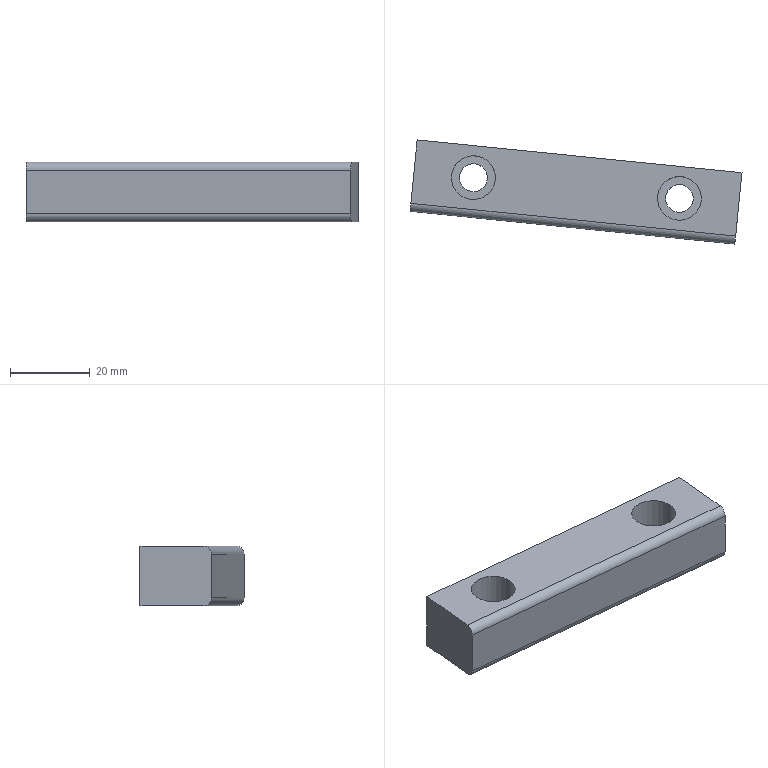Part | NX | features solid 2 | 1 solid | 14 faces | box 83.391 x 26.126 x 15 mm | volume 19827 mm3 | plane 8 | cylinder 6 | commonest cylinder face diameters 4 x2 7 x2 11 x2
STEP:
#1=CARTESIAN_POINT('',(735.965,124.652,-12.));
#2=VERTEX_POINT('',#1);
#3=CARTESIAN_POINT('',(734.362,108.732,-12.));
#4=VERTEX_POINT('',#3);
#5=CARTESIAN_POINT('',(735.164,116.692,-12.));
#6=DIRECTION('',(-0.1002,-0.995,0.));
#7=VECTOR('',#6,1000.);
#8=LINE('',#5,#7);
#9=EDGE_CURVE('',#2,#4,#8,.T.);
#10=ORIENTED_EDGE('',*,*,#9,.T.);
#11=CARTESIAN_POINT('',(652.775,116.948,-12.));
#12=VERTEX_POINT('',#11);
#13=CARTESIAN_POINT('',(646.805,117.549,-12.));
#14=DIRECTION('',(-0.995,0.1002,0.));
#15=VECTOR('',#14,1000.);
#16=LINE('',#13,#15);
#17=EDGE_CURVE('',#4,#12,#16,.T.);
#18=ORIENTED_EDGE('',*,*,#17,.T.);
#19=CARTESIAN_POINT('',(654.378,132.868,-12.));
#20=VERTEX_POINT('',#19);
#21=CARTESIAN_POINT('',(653.576,124.908,-12.));
#22=DIRECTION('',(-0.1002,-0.995,0.));
#23=VECTOR('',#22,1000.);
#24=LINE('',#21,#23);
#25=EDGE_CURVE('',#20,#12,#24,.T.);
#26=ORIENTED_EDGE('',*,*,#25,.F.);
#27=CARTESIAN_POINT('',(648.408,133.469,-12.));
#28=DIRECTION('',(-0.995,0.1002,0.));
#29=VECTOR('',#28,1000.);
#30=LINE('',#27,#29);
#31=EDGE_CURVE('',#2,#20,#30,.T.);
#32=ORIENTED_EDGE('',*,*,#31,.F.);
#33=EDGE_LOOP('',(#10,#18,#26,#32));
#34=FACE_BOUND('',#33,.T.);
#35=CARTESIAN_POINT('',(716.766,118.627,-12.));
#36=VERTEX_POINT('',#35);
#37=CARTESIAN_POINT('',(720.239,118.195,-12.));
#38=DIRECTION('',(0.,0.,1.));
#39=DIRECTION('',(-0.9923,0.1236,0.));
#40=AXIS2_PLACEMENT_3D('',#37,#38,#39);
#41=CIRCLE('',#40,3.5);
#42=EDGE_CURVE('',#36,#36,#41,.T.);
#43=ORIENTED_EDGE('',*,*,#42,.T.);
#44=EDGE_LOOP('',(#43));
#45=FACE_BOUND('',#44,.T.);
#46=CARTESIAN_POINT('',(671.99,123.136,-12.));
#47=VERTEX_POINT('',#46);
#48=CARTESIAN_POINT('',(668.501,123.405,-12.));
#49=DIRECTION('',(0.,0.,-1.));
#50=DIRECTION('',(0.997,-0.07676,0.));
#51=AXIS2_PLACEMENT_3D('',#48,#49,#50);
#52=CIRCLE('',#51,3.5);
#53=EDGE_CURVE('',#47,#47,#52,.T.);
#54=ORIENTED_EDGE('',*,*,#53,.F.);
#55=EDGE_LOOP('',(#54));
#56=FACE_BOUND('',#55,.T.);
#57=CARTESIAN_POINT('',(647.606,125.509,-12.));
#58=DIRECTION('',(0.,0.,1.));
#59=DIRECTION('',(-0.9923,0.1236,0.));
#60=AXIS2_PLACEMENT_3D('',#57,#58,#59);
#61=PLANE('',#60);
#62=ADVANCED_FACE('',(#34,#45,#56),#61,.F.);
#63=CARTESIAN_POINT('',(654.378,132.868,3.));
#64=VERTEX_POINT('',#63);
#65=CARTESIAN_POINT('',(652.775,116.948,3.));
#66=VERTEX_POINT('',#65);
#67=CARTESIAN_POINT('',(653.576,124.908,3.));
#68=DIRECTION('',(-0.1002,-0.995,0.));
#69=VECTOR('',#68,1000.);
#70=LINE('',#67,#69);
#71=EDGE_CURVE('',#64,#66,#70,.T.);
#72=ORIENTED_EDGE('',*,*,#71,.T.);
#73=CARTESIAN_POINT('',(734.362,108.732,3.));
#74=VERTEX_POINT('',#73);
#75=CARTESIAN_POINT('',(646.805,117.549,3.));
#76=DIRECTION('',(0.995,-0.1002,0.));
#77=VECTOR('',#76,1000.);
#78=LINE('',#75,#77);
#79=EDGE_CURVE('',#66,#74,#78,.T.);
#80=ORIENTED_EDGE('',*,*,#79,.T.);
#81=CARTESIAN_POINT('',(735.965,124.652,3.));
#82=VERTEX_POINT('',#81);
#83=CARTESIAN_POINT('',(735.164,116.692,3.));
#84=DIRECTION('',(-0.1002,-0.995,0.));
#85=VECTOR('',#84,1000.);
#86=LINE('',#83,#85);
#87=EDGE_CURVE('',#82,#74,#86,.T.);
#88=ORIENTED_EDGE('',*,*,#87,.F.);
#89=CARTESIAN_POINT('',(648.408,133.469,3.));
#90=DIRECTION('',(0.995,-0.1002,0.));
#91=VECTOR('',#90,1000.);
#92=LINE('',#89,#91);
#93=EDGE_CURVE('',#64,#82,#92,.T.);
#94=ORIENTED_EDGE('',*,*,#93,.F.);
#95=EDGE_LOOP('',(#72,#80,#88,#94));
#96=FACE_BOUND('',#95,.T.);
#97=CARTESIAN_POINT('',(714.781,118.874,3.));
#98=VERTEX_POINT('',#97);
#99=CARTESIAN_POINT('',(720.239,118.195,3.));
#100=DIRECTION('',(0.,0.,-1.));
#101=DIRECTION('',(-0.9923,0.1236,0.));
#102=AXIS2_PLACEMENT_3D('',#99,#100,#101);
#103=CIRCLE('',#102,5.5);
#104=EDGE_CURVE('',#98,#98,#103,.T.);
#105=ORIENTED_EDGE('',*,*,#104,.T.);
#106=EDGE_LOOP('',(#105));
#107=FACE_BOUND('',#106,.T.);
#108=CARTESIAN_POINT('',(673.985,122.983,3.));
#109=VERTEX_POINT('',#108);
#110=CARTESIAN_POINT('',(668.501,123.405,3.));
#111=DIRECTION('',(0.,0.,1.));
#112=DIRECTION('',(0.997,-0.07676,0.));
#113=AXIS2_PLACEMENT_3D('',#110,#111,#112);
#114=CIRCLE('',#113,5.5);
#115=EDGE_CURVE('',#109,#109,#114,.T.);
#116=ORIENTED_EDGE('',*,*,#115,.F.);
#117=EDGE_LOOP('',(#116));
#118=FACE_BOUND('',#117,.T.);
#119=CARTESIAN_POINT('',(647.606,125.509,3.));
#120=DIRECTION('',(0.,0.,-1.));
#121=DIRECTION('',(0.9923,-0.1236,0.));
#122=AXIS2_PLACEMENT_3D('',#119,#120,#121);
#123=PLANE('',#122);
#124=ADVANCED_FACE('',(#96,#107,#118),#123,.F.);
#125=CARTESIAN_POINT('',(734.162,106.742,1.));
#126=VERTEX_POINT('',#125);
#127=CARTESIAN_POINT('',(734.162,106.742,-10.));
#128=VERTEX_POINT('',#127);
#129=CARTESIAN_POINT('',(734.162,106.742,50.));
#130=DIRECTION('',(0.,0.,-1.));
#131=VECTOR('',#130,1000.);
#132=LINE('',#129,#131);
#133=EDGE_CURVE('',#126,#128,#132,.T.);
#134=ORIENTED_EDGE('',*,*,#133,.T.);
#135=CARTESIAN_POINT('',(734.362,108.732,-10.));
#136=DIRECTION('',(-0.995,0.1002,0.));
#137=DIRECTION('',(-0.1002,-0.995,0.));
#138=AXIS2_PLACEMENT_3D('',#135,#136,#137);
#139=CIRCLE('',#138,2.);
#140=EDGE_CURVE('',#128,#4,#139,.F.);
#141=ORIENTED_EDGE('',*,*,#140,.T.);
#142=ORIENTED_EDGE('',*,*,#9,.F.);
#143=CARTESIAN_POINT('',(735.965,124.652,50.));
#144=DIRECTION('',(0.,0.,-1.));
#145=VECTOR('',#144,1000.);
#146=LINE('',#143,#145);
#147=EDGE_CURVE('',#82,#2,#146,.T.);
#148=ORIENTED_EDGE('',*,*,#147,.F.);
#149=ORIENTED_EDGE('',*,*,#87,.T.);
#150=CARTESIAN_POINT('',(734.362,108.732,1.));
#151=DIRECTION('',(-0.995,0.1002,0.));
#152=DIRECTION('',(-0.1002,-0.995,0.));
#153=AXIS2_PLACEMENT_3D('',#150,#151,#152);
#154=CIRCLE('',#153,2.);
#155=EDGE_CURVE('',#74,#126,#154,.F.);
#156=ORIENTED_EDGE('',*,*,#155,.T.);
#157=EDGE_LOOP('',(#134,#141,#142,#148,#149,#156));
#158=FACE_BOUND('',#157,.T.);
#159=CARTESIAN_POINT('',(735.164,116.692,50.));
#160=DIRECTION('',(-0.995,0.1002,0.));
#161=DIRECTION('',(-0.1002,-0.995,0.));
#162=AXIS2_PLACEMENT_3D('',#159,#160,#161);
#163=PLANE('',#162);
#164=ADVANCED_FACE('',(#158),#163,.F.);
#165=ORIENTED_EDGE('',*,*,#25,.T.);
#166=CARTESIAN_POINT('',(652.574,114.958,-10.));
#167=VERTEX_POINT('',#166);
#168=CARTESIAN_POINT('',(652.775,116.948,-10.));
#169=DIRECTION('',(0.995,-0.1002,0.));
#170=DIRECTION('',(0.1002,0.995,0.));
#171=AXIS2_PLACEMENT_3D('',#168,#169,#170);
#172=CIRCLE('',#171,2.);
#173=EDGE_CURVE('',#12,#167,#172,.F.);
#174=ORIENTED_EDGE('',*,*,#173,.T.);
#175=CARTESIAN_POINT('',(652.574,114.958,1.));
#176=VERTEX_POINT('',#175);
#177=CARTESIAN_POINT('',(652.574,114.958,50.));
#178=DIRECTION('',(0.,0.,1.));
#179=VECTOR('',#178,1000.);
#180=LINE('',#177,#179);
#181=EDGE_CURVE('',#167,#176,#180,.T.);
#182=ORIENTED_EDGE('',*,*,#181,.T.);
#183=CARTESIAN_POINT('',(652.775,116.948,1.));
#184=DIRECTION('',(0.995,-0.1002,0.));
#185=DIRECTION('',(0.1002,0.995,0.));
#186=AXIS2_PLACEMENT_3D('',#183,#184,#185);
#187=CIRCLE('',#186,2.);
#188=EDGE_CURVE('',#176,#66,#187,.F.);
#189=ORIENTED_EDGE('',*,*,#188,.T.);
#190=ORIENTED_EDGE('',*,*,#71,.F.);
#191=CARTESIAN_POINT('',(654.378,132.868,50.));
#192=DIRECTION('',(0.,0.,1.));
#193=VECTOR('',#192,1000.);
#194=LINE('',#191,#193);
#195=EDGE_CURVE('',#20,#64,#194,.T.);
#196=ORIENTED_EDGE('',*,*,#195,.F.);
#197=EDGE_LOOP('',(#165,#174,#182,#189,#190,#196));
#198=FACE_BOUND('',#197,.T.);
#199=CARTESIAN_POINT('',(653.576,124.908,50.));
#200=DIRECTION('',(0.995,-0.1002,0.));
#201=DIRECTION('',(0.1002,0.995,0.));
#202=AXIS2_PLACEMENT_3D('',#199,#200,#201);
#203=PLANE('',#202);
#204=ADVANCED_FACE('',(#198),#203,.F.);
#205=ORIENTED_EDGE('',*,*,#147,.T.);
#206=ORIENTED_EDGE('',*,*,#31,.T.);
#207=ORIENTED_EDGE('',*,*,#195,.T.);
#208=ORIENTED_EDGE('',*,*,#93,.T.);
#209=EDGE_LOOP('',(#205,#206,#207,#208));
#210=FACE_BOUND('',#209,.T.);
#211=CARTESIAN_POINT('',(648.408,133.469,50.));
#212=DIRECTION('',(0.1002,0.995,0.));
#213=DIRECTION('',(-0.995,0.1002,0.));
#214=AXIS2_PLACEMENT_3D('',#211,#212,#213);
#215=PLANE('',#214);
#216=ADVANCED_FACE('',(#210),#215,.T.);
#217=ORIENTED_EDGE('',*,*,#181,.F.);
#218=CARTESIAN_POINT('',(646.604,115.56,-10.));
#219=DIRECTION('',(-0.995,0.1002,0.));
#220=VECTOR('',#219,1000.);
#221=LINE('',#218,#220);
#222=EDGE_CURVE('',#167,#128,#221,.F.);
#223=ORIENTED_EDGE('',*,*,#222,.T.);
#224=ORIENTED_EDGE('',*,*,#133,.F.);
#225=CARTESIAN_POINT('',(646.604,115.56,1.));
#226=DIRECTION('',(0.995,-0.1002,0.));
#227=VECTOR('',#226,1000.);
#228=LINE('',#225,#227);
#229=EDGE_CURVE('',#126,#176,#228,.F.);
#230=ORIENTED_EDGE('',*,*,#229,.T.);
#231=EDGE_LOOP('',(#217,#223,#224,#230));
#232=FACE_BOUND('',#231,.T.);
#233=CARTESIAN_POINT('',(646.604,115.56,50.));
#234=DIRECTION('',(0.1002,0.995,0.));
#235=DIRECTION('',(-0.995,0.1002,0.));
#236=AXIS2_PLACEMENT_3D('',#233,#234,#235);
#237=PLANE('',#236);
#238=ADVANCED_FACE('',(#232),#237,.F.);
#239=ORIENTED_EDGE('',*,*,#140,.F.);
#240=ORIENTED_EDGE('',*,*,#222,.F.);
#241=ORIENTED_EDGE('',*,*,#173,.F.);
#242=ORIENTED_EDGE('',*,*,#17,.F.);
#243=EDGE_LOOP('',(#239,#240,#241,#242));
#244=FACE_BOUND('',#243,.T.);
#245=CARTESIAN_POINT('',(646.805,117.549,-10.));
#246=DIRECTION('',(-0.995,0.1002,0.));
#247=DIRECTION('',(-0.1002,-0.995,0.));
#248=AXIS2_PLACEMENT_3D('',#245,#246,#247);
#249=CYLINDRICAL_SURFACE('',#248,2.);
#250=ADVANCED_FACE('',(#244),#249,.T.);
#251=ORIENTED_EDGE('',*,*,#188,.F.);
#252=ORIENTED_EDGE('',*,*,#229,.F.);
#253=ORIENTED_EDGE('',*,*,#155,.F.);
#254=ORIENTED_EDGE('',*,*,#79,.F.);
#255=EDGE_LOOP('',(#251,#252,#253,#254));
#256=FACE_BOUND('',#255,.T.);
#257=CARTESIAN_POINT('',(646.805,117.549,1.));
#258=DIRECTION('',(0.995,-0.1002,0.));
#259=DIRECTION('',(0.1002,0.995,0.));
#260=AXIS2_PLACEMENT_3D('',#257,#258,#259);
#261=CYLINDRICAL_SURFACE('',#260,2.);
#262=ADVANCED_FACE('',(#256),#261,.T.);
#263=CARTESIAN_POINT('',(723.712,117.762,-6.));
#264=VERTEX_POINT('',#263);
#265=CARTESIAN_POINT('',(720.239,118.195,-6.));
#266=DIRECTION('',(0.,0.,-1.));
#267=DIRECTION('',(0.9923,-0.1236,0.));
#268=AXIS2_PLACEMENT_3D('',#265,#266,#267);
#269=CIRCLE('',#268,3.5);
#270=EDGE_CURVE('',#264,#264,#269,.T.);
#271=ORIENTED_EDGE('',*,*,#270,.F.);
#272=EDGE_LOOP('',(#271));
#273=FACE_BOUND('',#272,.T.);
#274=ORIENTED_EDGE('',*,*,#42,.F.);
#275=EDGE_LOOP('',(#274));
#276=FACE_BOUND('',#275,.T.);
#277=CARTESIAN_POINT('',(720.239,118.195,3.));
#278=DIRECTION('',(0.,0.,-1.));
#279=DIRECTION('',(-0.9923,0.1236,0.));
#280=AXIS2_PLACEMENT_3D('',#277,#278,#279);
#281=CYLINDRICAL_SURFACE('',#280,3.5);
#282=ADVANCED_FACE('',(#273,#276),#281,.F.);
#283=ORIENTED_EDGE('',*,*,#270,.T.);
#284=EDGE_LOOP('',(#283));
#285=FACE_BOUND('',#284,.T.);
#286=CARTESIAN_POINT('',(714.781,118.874,-6.));
#287=VERTEX_POINT('',#286);
#288=CARTESIAN_POINT('',(720.239,118.195,-6.));
#289=DIRECTION('',(0.,0.,1.));
#290=DIRECTION('',(-0.9923,0.1236,0.));
#291=AXIS2_PLACEMENT_3D('',#288,#289,#290);
#292=CIRCLE('',#291,5.5);
#293=EDGE_CURVE('',#287,#287,#292,.F.);
#294=ORIENTED_EDGE('',*,*,#293,.F.);
#295=EDGE_LOOP('',(#294));
#296=FACE_BOUND('',#295,.T.);
#297=CARTESIAN_POINT('',(720.239,118.195,-6.));
#298=DIRECTION('',(0.,0.,-1.));
#299=DIRECTION('',(0.9923,-0.1236,0.));
#300=AXIS2_PLACEMENT_3D('',#297,#298,#299);
#301=PLANE('',#300);
#302=ADVANCED_FACE('',(#285,#296),#301,.F.);
#303=ORIENTED_EDGE('',*,*,#293,.T.);
#304=EDGE_LOOP('',(#303));
#305=FACE_BOUND('',#304,.T.);
#306=ORIENTED_EDGE('',*,*,#104,.F.);
#307=EDGE_LOOP('',(#306));
#308=FACE_BOUND('',#307,.T.);
#309=CARTESIAN_POINT('',(720.239,118.195,3.));
#310=DIRECTION('',(0.,0.,-1.));
#311=DIRECTION('',(-0.9923,0.1236,0.));
#312=AXIS2_PLACEMENT_3D('',#309,#310,#311);
#313=CYLINDRICAL_SURFACE('',#312,5.5);
#314=ADVANCED_FACE('',(#305,#308),#313,.F.);
#315=CARTESIAN_POINT('',(665.011,123.674,-6.));
#316=VERTEX_POINT('',#315);
#317=CARTESIAN_POINT('',(668.501,123.405,-6.));
#318=DIRECTION('',(0.,0.,1.));
#319=DIRECTION('',(-0.997,0.07676,0.));
#320=AXIS2_PLACEMENT_3D('',#317,#318,#319);
#321=CIRCLE('',#320,3.5);
#322=EDGE_CURVE('',#316,#316,#321,.T.);
#323=ORIENTED_EDGE('',*,*,#322,.T.);
#324=EDGE_LOOP('',(#323));
#325=FACE_BOUND('',#324,.T.);
#326=ORIENTED_EDGE('',*,*,#53,.T.);
#327=EDGE_LOOP('',(#326));
#328=FACE_BOUND('',#327,.T.);
#329=CARTESIAN_POINT('',(668.501,123.405,3.));
#330=DIRECTION('',(0.,0.,-1.));
#331=DIRECTION('',(0.997,-0.07676,0.));
#332=AXIS2_PLACEMENT_3D('',#329,#330,#331);
#333=CYLINDRICAL_SURFACE('',#332,3.5);
#334=ADVANCED_FACE('',(#325,#328),#333,.F.);
#335=ORIENTED_EDGE('',*,*,#322,.F.);
#336=EDGE_LOOP('',(#335));
#337=FACE_BOUND('',#336,.T.);
#338=CARTESIAN_POINT('',(673.985,122.983,-6.));
#339=VERTEX_POINT('',#338);
#340=CARTESIAN_POINT('',(668.501,123.405,-6.));
#341=DIRECTION('',(0.,0.,-1.));
#342=DIRECTION('',(0.997,-0.07676,0.));
#343=AXIS2_PLACEMENT_3D('',#340,#341,#342);
#344=CIRCLE('',#343,5.5);
#345=EDGE_CURVE('',#339,#339,#344,.F.);
#346=ORIENTED_EDGE('',*,*,#345,.T.);
#347=EDGE_LOOP('',(#346));
#348=FACE_BOUND('',#347,.T.);
#349=CARTESIAN_POINT('',(668.501,123.405,-6.));
#350=DIRECTION('',(0.,0.,-1.));
#351=DIRECTION('',(-0.997,0.07676,0.));
#352=AXIS2_PLACEMENT_3D('',#349,#350,#351);
#353=PLANE('',#352);
#354=ADVANCED_FACE('',(#337,#348),#353,.F.);
#355=ORIENTED_EDGE('',*,*,#345,.F.);
#356=EDGE_LOOP('',(#355));
#357=FACE_BOUND('',#356,.T.);
#358=ORIENTED_EDGE('',*,*,#115,.T.);
#359=EDGE_LOOP('',(#358));
#360=FACE_BOUND('',#359,.T.);
#361=CARTESIAN_POINT('',(668.501,123.405,3.));
#362=DIRECTION('',(0.,0.,-1.));
#363=DIRECTION('',(0.997,-0.07676,0.));
#364=AXIS2_PLACEMENT_3D('',#361,#362,#363);
#365=CYLINDRICAL_SURFACE('',#364,5.5);
#366=ADVANCED_FACE('',(#357,#360),#365,.F.);
#367=CLOSED_SHELL('',(#62,#124,#164,#204,#216,#238,#250,#262,#282,#302,#314,#334,#354,#366));
#368=MANIFOLD_SOLID_BREP('',#367);
#369=(LENGTH_UNIT()NAMED_UNIT(*)SI_UNIT(.MILLI.,.METRE.));
#370=UNCERTAINTY_MEASURE_WITH_UNIT(LENGTH_MEASURE(0.00001),#369,'','');
#371=(NAMED_UNIT(*)PLANE_ANGLE_UNIT()SI_UNIT($,.RADIAN.));
#372=(NAMED_UNIT(*)SI_UNIT($,.STERADIAN.)SOLID_ANGLE_UNIT());
#373=(GEOMETRIC_REPRESENTATION_CONTEXT(3)GLOBAL_UNCERTAINTY_ASSIGNED_CONTEXT((#370))GLOBAL_UNIT_ASSIGNED_CONTEXT((#369,#371,#372))REPRESENTATION_CONTEXT('',''));
#374=ADVANCED_BREP_SHAPE_REPRESENTATION('',(#368),#373);